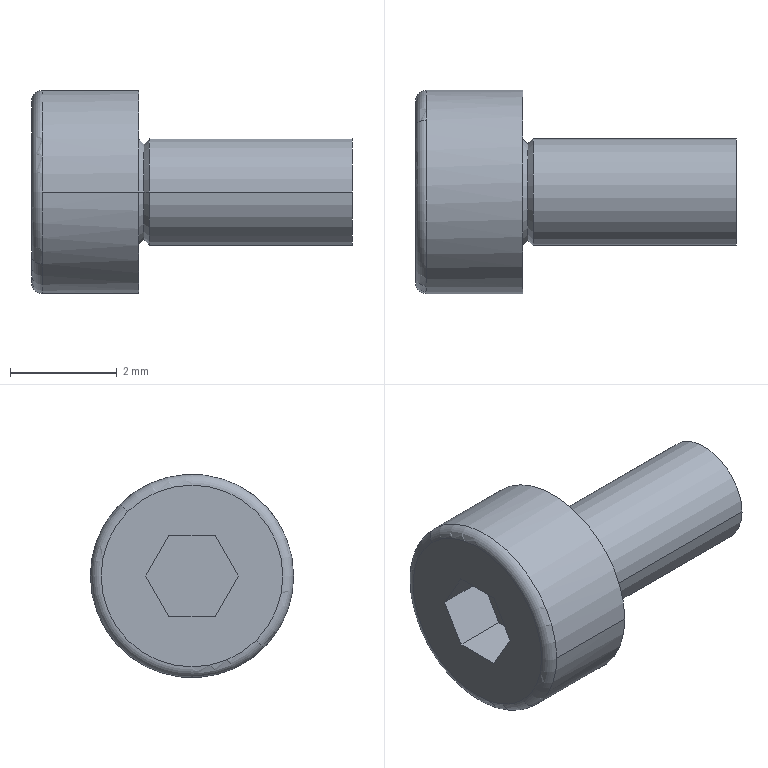Part | STEP file | ASND-0110-0211110210 | 1 solid | 20 faces | box 6 x 3.8 x 3.8 mm | volume 33.139 mm3 | plane 10 | cylinder 4 | cone 4 | torus 2 | commonest cylinder face diameters 2 x2 3.8 x2
STEP:
#1=CARTESIAN_POINT('',(0.,0.,0.));
#2=DIRECTION('',(0.,0.,1.));
#3=DIRECTION('',(1.,0.,0.));
#4=AXIS2_PLACEMENT_3D('',#1,#2,#3);
#5=CARTESIAN_POINT('',(-2.,-1.202,-1.202));
#6=VERTEX_POINT('',#5);
#7=CARTESIAN_POINT('',(-2.,1.202,1.202));
#8=VERTEX_POINT('',#7);
#9=CARTESIAN_POINT('',(-2.,0.,0.));
#10=DIRECTION('',(-1.,0.,0.));
#11=DIRECTION('',(0.,-1.,0.));
#12=AXIS2_PLACEMENT_3D('',#9,#10,#11);
#13=CIRCLE('',#12,1.7);
#14=CARTESIAN_POINT('',(-1.8,0.,0.));
#15=DIRECTION('',(1.,0.,0.));
#16=DIRECTION('',(0.,0.7071,0.7071));
#17=AXIS2_PLACEMENT_3D('',#14,#15,#16);
#18=TOROIDAL_SURFACE('',#17,1.7,0.2);
#19=CARTESIAN_POINT('',(8.639,4.712));
#20=DIRECTION('',(-1.,0.));
#21=VECTOR('',#20,1.);
#22=LINE('',#19,#21);
#23=(GEOMETRIC_REPRESENTATION_CONTEXT(2)PARAMETRIC_REPRESENTATION_CONTEXT()REPRESENTATION_CONTEXT('',''));
#24=DEFINITIONAL_REPRESENTATION('',(#22),#23);
#25=PCURVE('',#18,#24);
#26=CARTESIAN_POINT('',(-2.,0.,0.));
#27=DIRECTION('',(1.,0.,0.));
#28=DIRECTION('',(0.,0.7071,0.7071));
#29=AXIS2_PLACEMENT_3D('',#26,#27,#28);
#30=PLANE('',#29);
#31=CARTESIAN_POINT('',(-1.202,1.202));
#32=CARTESIAN_POINT('',(0.88,3.284));
#33=CARTESIAN_POINT('',(1.642,0.44));
#34=CARTESIAN_POINT('',(2.404,-2.404));
#35=CARTESIAN_POINT('',(-0.44,-1.642));
#36=CARTESIAN_POINT('',(-3.284,-0.88));
#37=CARTESIAN_POINT('',(-1.202,1.202));
#38=(BOUNDED_CURVE()B_SPLINE_CURVE(2,(#31,#32,#33,#34,#35,#36,#37),.UNSPECIFIED.,.T.,.F.)B_SPLINE_CURVE_WITH_KNOTS((1,2,2,2,2,1),(-2.094,0.,2.094,4.189,6.283,8.378),.UNSPECIFIED.)CURVE()GEOMETRIC_REPRESENTATION_ITEM()RATIONAL_B_SPLINE_CURVE((1.,0.5,1.,0.5,1.,0.5,1.))REPRESENTATION_ITEM(''));
#39=(GEOMETRIC_REPRESENTATION_CONTEXT(2)PARAMETRIC_REPRESENTATION_CONTEXT()REPRESENTATION_CONTEXT('',''));
#40=DEFINITIONAL_REPRESENTATION('',(#38),#39);
#41=PCURVE('',#30,#40);
#42=SURFACE_CURVE('',#13,(#25,#41),.PCURVE_S1.);
#43=EDGE_CURVE('',#6,#8,#42,.T.);
#44=ORIENTED_EDGE('',*,*,#43,.F.);
#45=CARTESIAN_POINT('',(-1.8,-1.344,-1.344));
#46=VERTEX_POINT('',#45);
#47=CARTESIAN_POINT('',(-1.8,-1.202,-1.202));
#48=DIRECTION('',(0.,-0.7071,0.7071));
#49=DIRECTION('',(0.,-0.7071,-0.7071));
#50=AXIS2_PLACEMENT_3D('',#47,#48,#49);
#51=CIRCLE('',#50,0.2);
#52=CARTESIAN_POINT('',(3.142,0.));
#53=DIRECTION('',(0.,1.));
#54=VECTOR('',#53,1.);
#55=LINE('',#52,#54);
#56=(GEOMETRIC_REPRESENTATION_CONTEXT(2)PARAMETRIC_REPRESENTATION_CONTEXT()REPRESENTATION_CONTEXT('',''));
#57=DEFINITIONAL_REPRESENTATION('',(#55),#56);
#58=PCURVE('',#18,#57);
#59=CARTESIAN_POINT('',(-1.8,0.,0.));
#60=DIRECTION('',(1.,0.,0.));
#61=DIRECTION('',(0.,0.7071,0.7071));
#62=AXIS2_PLACEMENT_3D('',#59,#60,#61);
#63=TOROIDAL_SURFACE('',#62,1.7,0.2);
#64=CARTESIAN_POINT('',(3.142,0.));
#65=DIRECTION('',(0.,1.));
#66=VECTOR('',#65,1.);
#67=LINE('',#64,#66);
#68=(GEOMETRIC_REPRESENTATION_CONTEXT(2)PARAMETRIC_REPRESENTATION_CONTEXT()REPRESENTATION_CONTEXT('',''));
#69=DEFINITIONAL_REPRESENTATION('',(#67),#68);
#70=PCURVE('',#63,#69);
#71=SURFACE_CURVE('',#51,(#58,#70),.PCURVE_S1.);
#72=EDGE_CURVE('',#6,#46,#71,.T.);
#73=ORIENTED_EDGE('',*,*,#72,.T.);
#74=CARTESIAN_POINT('',(-1.8,-1.9,0.));
#75=VERTEX_POINT('',#74);
#76=CARTESIAN_POINT('',(-1.8,0.,0.));
#77=DIRECTION('',(-1.,0.,0.));
#78=DIRECTION('',(0.,-1.,0.));
#79=AXIS2_PLACEMENT_3D('',#76,#77,#78);
#80=CIRCLE('',#79,1.9);
#81=CARTESIAN_POINT('',(8.639,6.283));
#82=DIRECTION('',(-1.,0.));
#83=VECTOR('',#82,1.);
#84=LINE('',#81,#83);
#85=(GEOMETRIC_REPRESENTATION_CONTEXT(2)PARAMETRIC_REPRESENTATION_CONTEXT()REPRESENTATION_CONTEXT('',''));
#86=DEFINITIONAL_REPRESENTATION('',(#84),#85);
#87=PCURVE('',#18,#86);
#88=CARTESIAN_POINT('',(-2.3,0.,0.));
#89=DIRECTION('',(1.,0.,0.));
#90=DIRECTION('',(0.,1.,0.));
#91=AXIS2_PLACEMENT_3D('',#88,#89,#90);
#92=CYLINDRICAL_SURFACE('',#91,1.9);
#93=CARTESIAN_POINT('',(9.425,0.5));
#94=DIRECTION('',(-1.,0.));
#95=VECTOR('',#94,1.);
#96=LINE('',#93,#95);
#97=(GEOMETRIC_REPRESENTATION_CONTEXT(2)PARAMETRIC_REPRESENTATION_CONTEXT()REPRESENTATION_CONTEXT('',''));
#98=DEFINITIONAL_REPRESENTATION('',(#96),#97);
#99=PCURVE('',#92,#98);
#100=SURFACE_CURVE('',#80,(#87,#99),.PCURVE_S1.);
#101=EDGE_CURVE('',#46,#75,#100,.T.);
#102=ORIENTED_EDGE('',*,*,#101,.T.);
#103=CARTESIAN_POINT('',(-1.8,1.344,1.344));
#104=VERTEX_POINT('',#103);
#105=CARTESIAN_POINT('',(-1.8,0.,0.));
#106=DIRECTION('',(-1.,0.,0.));
#107=DIRECTION('',(0.,-1.,0.));
#108=AXIS2_PLACEMENT_3D('',#105,#106,#107);
#109=CIRCLE('',#108,1.9);
#110=CARTESIAN_POINT('',(2.356,6.283));
#111=DIRECTION('',(-1.,0.));
#112=VECTOR('',#111,1.);
#113=LINE('',#110,#112);
#114=(GEOMETRIC_REPRESENTATION_CONTEXT(2)PARAMETRIC_REPRESENTATION_CONTEXT()REPRESENTATION_CONTEXT('',''));
#115=DEFINITIONAL_REPRESENTATION('',(#113),#114);
#116=PCURVE('',#18,#115);
#117=CARTESIAN_POINT('',(-2.3,0.,0.));
#118=DIRECTION('',(1.,0.,0.));
#119=DIRECTION('',(0.,1.,0.));
#120=AXIS2_PLACEMENT_3D('',#117,#118,#119);
#121=CYLINDRICAL_SURFACE('',#120,1.9);
#122=CARTESIAN_POINT('',(3.142,0.5));
#123=DIRECTION('',(-1.,0.));
#124=VECTOR('',#123,1.);
#125=LINE('',#122,#124);
#126=(GEOMETRIC_REPRESENTATION_CONTEXT(2)PARAMETRIC_REPRESENTATION_CONTEXT()REPRESENTATION_CONTEXT('',''));
#127=DEFINITIONAL_REPRESENTATION('',(#125),#126);
#128=PCURVE('',#121,#127);
#129=SURFACE_CURVE('',#109,(#116,#128),.PCURVE_S1.);
#130=EDGE_CURVE('',#75,#104,#129,.T.);
#131=ORIENTED_EDGE('',*,*,#130,.T.);
#132=CARTESIAN_POINT('',(-1.8,1.202,1.202));
#133=DIRECTION('',(0.,0.7071,-0.7071));
#134=DIRECTION('',(0.,0.7071,0.7071));
#135=AXIS2_PLACEMENT_3D('',#132,#133,#134);
#136=CIRCLE('',#135,0.2);
#137=CARTESIAN_POINT('',(0.,0.));
#138=DIRECTION('',(0.,1.));
#139=VECTOR('',#138,1.);
#140=LINE('',#137,#139);
#141=(GEOMETRIC_REPRESENTATION_CONTEXT(2)PARAMETRIC_REPRESENTATION_CONTEXT()REPRESENTATION_CONTEXT('',''));
#142=DEFINITIONAL_REPRESENTATION('',(#140),#141);
#143=PCURVE('',#18,#142);
#144=CARTESIAN_POINT('',(6.283,0.));
#145=DIRECTION('',(0.,1.));
#146=VECTOR('',#145,1.);
#147=LINE('',#144,#146);
#148=(GEOMETRIC_REPRESENTATION_CONTEXT(2)PARAMETRIC_REPRESENTATION_CONTEXT()REPRESENTATION_CONTEXT('',''));
#149=DEFINITIONAL_REPRESENTATION('',(#147),#148);
#150=PCURVE('',#63,#149);
#151=SURFACE_CURVE('',#136,(#143,#150),.PCURVE_S1.);
#152=EDGE_CURVE('',#8,#104,#151,.T.);
#153=ORIENTED_EDGE('',*,*,#152,.F.);
#154=EDGE_LOOP('',(#44,#73,#102,#131,#153));
#155=FACE_BOUND('',#154,.T.);
#156=ADVANCED_FACE('',(#155),#18,.T.);
#157=ORIENTED_EDGE('',*,*,#130,.F.);
#158=CARTESIAN_POINT('',(0.,-1.9,0.));
#159=VERTEX_POINT('',#158);
#160=CARTESIAN_POINT('',(-2.3,-1.9,0.));
#161=DIRECTION('',(1.,0.,0.));
#162=VECTOR('',#161,1.);
#163=LINE('',#160,#162);
#164=CARTESIAN_POINT('',(3.142,0.));
#165=DIRECTION('',(0.,1.));
#166=VECTOR('',#165,1.);
#167=LINE('',#164,#166);
#168=(GEOMETRIC_REPRESENTATION_CONTEXT(2)PARAMETRIC_REPRESENTATION_CONTEXT()REPRESENTATION_CONTEXT('',''));
#169=DEFINITIONAL_REPRESENTATION('',(#167),#168);
#170=PCURVE('',#121,#169);
#171=CARTESIAN_POINT('',(3.142,0.));
#172=DIRECTION('',(0.,1.));
#173=VECTOR('',#172,1.);
#174=LINE('',#171,#173);
#175=(GEOMETRIC_REPRESENTATION_CONTEXT(2)PARAMETRIC_REPRESENTATION_CONTEXT()REPRESENTATION_CONTEXT('',''));
#176=DEFINITIONAL_REPRESENTATION('',(#174),#175);
#177=PCURVE('',#92,#176);
#178=SURFACE_CURVE('',#163,(#170,#177),.PCURVE_S1.);
#179=EDGE_CURVE('',#75,#159,#178,.T.);
#180=ORIENTED_EDGE('',*,*,#179,.T.);
#181=CARTESIAN_POINT('',(0.,1.9,0.));
#182=VERTEX_POINT('',#181);
#183=CARTESIAN_POINT('',(0.,0.,0.));
#184=DIRECTION('',(-1.,0.,0.));
#185=DIRECTION('',(0.,-1.,0.));
#186=AXIS2_PLACEMENT_3D('',#183,#184,#185);
#187=CIRCLE('',#186,1.9);
#188=CARTESIAN_POINT('',(3.142,2.3));
#189=DIRECTION('',(-1.,0.));
#190=VECTOR('',#189,1.);
#191=LINE('',#188,#190);
#192=(GEOMETRIC_REPRESENTATION_CONTEXT(2)PARAMETRIC_REPRESENTATION_CONTEXT()REPRESENTATION_CONTEXT('',''));
#193=DEFINITIONAL_REPRESENTATION('',(#191),#192);
#194=PCURVE('',#121,#193);
#195=CARTESIAN_POINT('',(0.,0.,0.));
#196=DIRECTION('',(1.,0.,0.));
#197=DIRECTION('',(0.,0.7071,0.7071));
#198=AXIS2_PLACEMENT_3D('',#195,#196,#197);
#199=PLANE('',#198);
#200=CARTESIAN_POINT('',(-1.344,1.344));
#201=CARTESIAN_POINT('',(0.9835,3.671));
#202=CARTESIAN_POINT('',(1.835,0.4918));
#203=CARTESIAN_POINT('',(2.687,-2.687));
#204=CARTESIAN_POINT('',(-0.4918,-1.835));
#205=CARTESIAN_POINT('',(-3.671,-0.9835));
#206=CARTESIAN_POINT('',(-1.344,1.344));
#207=(BOUNDED_CURVE()B_SPLINE_CURVE(2,(#200,#201,#202,#203,#204,#205,#206),.UNSPECIFIED.,.T.,.F.)B_SPLINE_CURVE_WITH_KNOTS((1,2,2,2,2,1),(-2.094,0.,2.094,4.189,6.283,8.378),.UNSPECIFIED.)CURVE()GEOMETRIC_REPRESENTATION_ITEM()RATIONAL_B_SPLINE_CURVE((1.,0.5,1.,0.5,1.,0.5,1.))REPRESENTATION_ITEM(''));
#208=(GEOMETRIC_REPRESENTATION_CONTEXT(2)PARAMETRIC_REPRESENTATION_CONTEXT()REPRESENTATION_CONTEXT('',''));
#209=DEFINITIONAL_REPRESENTATION('',(#207),#208);
#210=PCURVE('',#199,#209);
#211=SURFACE_CURVE('',#187,(#194,#210),.PCURVE_S1.);
#212=EDGE_CURVE('',#159,#182,#211,.T.);
#213=ORIENTED_EDGE('',*,*,#212,.T.);
#214=CARTESIAN_POINT('',(-1.8,1.9,0.));
#215=VERTEX_POINT('',#214);
#216=CARTESIAN_POINT('',(-2.3,1.9,0.));
#217=DIRECTION('',(1.,0.,0.));
#218=VECTOR('',#217,1.);
#219=LINE('',#216,#218);
#220=CARTESIAN_POINT('',(0.,0.));
#221=DIRECTION('',(0.,1.));
#222=VECTOR('',#221,1.);
#223=LINE('',#220,#222);
#224=(GEOMETRIC_REPRESENTATION_CONTEXT(2)PARAMETRIC_REPRESENTATION_CONTEXT()REPRESENTATION_CONTEXT('',''));
#225=DEFINITIONAL_REPRESENTATION('',(#223),#224);
#226=PCURVE('',#121,#225);
#227=CARTESIAN_POINT('',(6.283,0.));
#228=DIRECTION('',(0.,1.));
#229=VECTOR('',#228,1.);
#230=LINE('',#227,#229);
#231=(GEOMETRIC_REPRESENTATION_CONTEXT(2)PARAMETRIC_REPRESENTATION_CONTEXT()REPRESENTATION_CONTEXT('',''));
#232=DEFINITIONAL_REPRESENTATION('',(#230),#231);
#233=PCURVE('',#92,#232);
#234=SURFACE_CURVE('',#219,(#226,#233),.PCURVE_S1.);
#235=EDGE_CURVE('',#215,#182,#234,.T.);
#236=ORIENTED_EDGE('',*,*,#235,.F.);
#237=CARTESIAN_POINT('',(-1.8,0.,0.));
#238=DIRECTION('',(-1.,0.,0.));
#239=DIRECTION('',(0.,-1.,0.));
#240=AXIS2_PLACEMENT_3D('',#237,#238,#239);
#241=CIRCLE('',#240,1.9);
#242=CARTESIAN_POINT('',(3.142,0.5));
#243=DIRECTION('',(-1.,0.));
#244=VECTOR('',#243,1.);
#245=LINE('',#242,#244);
#246=(GEOMETRIC_REPRESENTATION_CONTEXT(2)PARAMETRIC_REPRESENTATION_CONTEXT()REPRESENTATION_CONTEXT('',''));
#247=DEFINITIONAL_REPRESENTATION('',(#245),#246);
#248=PCURVE('',#121,#247);
#249=CARTESIAN_POINT('',(8.639,6.283));
#250=DIRECTION('',(-1.,0.));
#251=VECTOR('',#250,1.);
#252=LINE('',#249,#251);
#253=(GEOMETRIC_REPRESENTATION_CONTEXT(2)PARAMETRIC_REPRESENTATION_CONTEXT()REPRESENTATION_CONTEXT('',''));
#254=DEFINITIONAL_REPRESENTATION('',(#252),#253);
#255=PCURVE('',#63,#254);
#256=SURFACE_CURVE('',#241,(#248,#255),.PCURVE_S1.);
#257=EDGE_CURVE('',#104,#215,#256,.T.);
#258=ORIENTED_EDGE('',*,*,#257,.F.);
#259=EDGE_LOOP('',(#157,#180,#213,#236,#258));
#260=FACE_BOUND('',#259,.T.);
#261=ADVANCED_FACE('',(#260),#121,.T.);
#262=CARTESIAN_POINT('',(0.1,-0.9,0.));
#263=VERTEX_POINT('',#262);
#264=CARTESIAN_POINT('',(0.1,0.9,0.));
#265=VERTEX_POINT('',#264);
#266=CARTESIAN_POINT('',(0.1,0.,0.));
#267=DIRECTION('',(1.,0.,0.));
#268=DIRECTION('',(0.,1.,0.));
#269=AXIS2_PLACEMENT_3D('',#266,#267,#268);
#270=CIRCLE('',#269,0.9);
#271=CARTESIAN_POINT('',(0.,0.,0.));
#272=DIRECTION('',(-1.,0.,0.));
#273=DIRECTION('',(0.,1.,0.));
#274=AXIS2_PLACEMENT_3D('',#271,#272,#273);
#275=CONICAL_SURFACE('',#274,1.,0.7854);
#276=CARTESIAN_POINT('',(6.283,-0.1));
#277=DIRECTION('',(-1.,0.));
#278=VECTOR('',#277,1.);
#279=LINE('',#276,#278);
#280=(GEOMETRIC_REPRESENTATION_CONTEXT(2)PARAMETRIC_REPRESENTATION_CONTEXT()REPRESENTATION_CONTEXT('',''));
#281=DEFINITIONAL_REPRESENTATION('',(#279),#280);
#282=PCURVE('',#275,#281);
#283=CARTESIAN_POINT('',(0.2,0.,0.));
#284=DIRECTION('',(1.,0.,0.));
#285=DIRECTION('',(0.,-1.,0.));
#286=AXIS2_PLACEMENT_3D('',#283,#284,#285);
#287=CONICAL_SURFACE('',#286,1.,0.7854);
#288=CARTESIAN_POINT('',(-3.142,-0.1));
#289=DIRECTION('',(1.,0.));
#290=VECTOR('',#289,1.);
#291=LINE('',#288,#290);
#292=(GEOMETRIC_REPRESENTATION_CONTEXT(2)PARAMETRIC_REPRESENTATION_CONTEXT()REPRESENTATION_CONTEXT('',''));
#293=DEFINITIONAL_REPRESENTATION('',(#291),#292);
#294=PCURVE('',#287,#293);
#295=SURFACE_CURVE('',#270,(#282,#294),.PCURVE_S1.);
#296=EDGE_CURVE('',#263,#265,#295,.T.);
#297=ORIENTED_EDGE('',*,*,#296,.F.);
#298=CARTESIAN_POINT('',(0.,-1.,0.));
#299=VERTEX_POINT('',#298);
#300=CARTESIAN_POINT('',(0.,-1.,0.));
#301=DIRECTION('',(-0.7071,-0.7071,0.));
#302=VECTOR('',#301,1.);
#303=LINE('',#300,#302);
#304=CARTESIAN_POINT('',(3.142,0.));
#305=DIRECTION('',(0.,1.));
#306=VECTOR('',#305,1.);
#307=LINE('',#304,#306);
#308=(GEOMETRIC_REPRESENTATION_CONTEXT(2)PARAMETRIC_REPRESENTATION_CONTEXT()REPRESENTATION_CONTEXT('',''));
#309=DEFINITIONAL_REPRESENTATION('',(#307),#308);
#310=PCURVE('',#275,#309);
#311=CARTESIAN_POINT('',(0.,0.,0.));
#312=DIRECTION('',(-1.,0.,0.));
#313=DIRECTION('',(0.,1.,0.));
#314=AXIS2_PLACEMENT_3D('',#311,#312,#313);
#315=CONICAL_SURFACE('',#314,1.,0.7854);
#316=CARTESIAN_POINT('',(3.142,0.));
#317=DIRECTION('',(0.,1.));
#318=VECTOR('',#317,1.);
#319=LINE('',#316,#318);
#320=(GEOMETRIC_REPRESENTATION_CONTEXT(2)PARAMETRIC_REPRESENTATION_CONTEXT()REPRESENTATION_CONTEXT('',''));
#321=DEFINITIONAL_REPRESENTATION('',(#319),#320);
#322=PCURVE('',#315,#321);
#323=SURFACE_CURVE('',#303,(#310,#322),.PCURVE_S1.);
#324=EDGE_CURVE('',#263,#299,#323,.T.);
#325=ORIENTED_EDGE('',*,*,#324,.T.);
#326=CARTESIAN_POINT('',(0.,1.,0.));
#327=VERTEX_POINT('',#326);
#328=CARTESIAN_POINT('',(0.,0.,0.));
#329=DIRECTION('',(1.,0.,0.));
#330=DIRECTION('',(0.,-1.,0.));
#331=AXIS2_PLACEMENT_3D('',#328,#329,#330);
#332=CIRCLE('',#331,1.);
#333=CARTESIAN_POINT('',(3.142,0.));
#334=DIRECTION('',(-1.,0.));
#335=VECTOR('',#334,1.);
#336=LINE('',#333,#335);
#337=(GEOMETRIC_REPRESENTATION_CONTEXT(2)PARAMETRIC_REPRESENTATION_CONTEXT()REPRESENTATION_CONTEXT('',''));
#338=DEFINITIONAL_REPRESENTATION('',(#336),#337);
#339=PCURVE('',#275,#338);
#340=CARTESIAN_POINT('',(0.,0.));
#341=DIRECTION('',(-0.7071,0.7071));
#342=AXIS2_PLACEMENT_2D('',#340,#341);
#343=CIRCLE('',#342,1.);
#344=(GEOMETRIC_REPRESENTATION_CONTEXT(2)PARAMETRIC_REPRESENTATION_CONTEXT()REPRESENTATION_CONTEXT('',''));
#345=DEFINITIONAL_REPRESENTATION('',(#343),#344);
#346=PCURVE('',#199,#345);
#347=SURFACE_CURVE('',#332,(#339,#346),.PCURVE_S1.);
#348=EDGE_CURVE('',#299,#327,#347,.T.);
#349=ORIENTED_EDGE('',*,*,#348,.T.);
#350=CARTESIAN_POINT('',(0.,1.,0.));
#351=DIRECTION('',(-0.7071,0.7071,0.));
#352=VECTOR('',#351,1.);
#353=LINE('',#350,#352);
#354=CARTESIAN_POINT('',(0.,0.));
#355=DIRECTION('',(0.,1.));
#356=VECTOR('',#355,1.);
#357=LINE('',#354,#356);
#358=(GEOMETRIC_REPRESENTATION_CONTEXT(2)PARAMETRIC_REPRESENTATION_CONTEXT()REPRESENTATION_CONTEXT('',''));
#359=DEFINITIONAL_REPRESENTATION('',(#357),#358);
#360=PCURVE('',#275,#359);
#361=CARTESIAN_POINT('',(6.283,0.));
#362=DIRECTION('',(0.,1.));
#363=VECTOR('',#362,1.);
#364=LINE('',#361,#363);
#365=(GEOMETRIC_REPRESENTATION_CONTEXT(2)PARAMETRIC_REPRESENTATION_CONTEXT()REPRESENTATION_CONTEXT('',''));
#366=DEFINITIONAL_REPRESENTATION('',(#364),#365);
#367=PCURVE('',#315,#366);
#368=SURFACE_CURVE('',#353,(#360,#367),.PCURVE_S1.);
#369=EDGE_CURVE('',#265,#327,#368,.T.);
#370=ORIENTED_EDGE('',*,*,#369,.F.);
#371=EDGE_LOOP('',(#297,#325,#349,#370));
#372=FACE_BOUND('',#371,.T.);
#373=ADVANCED_FACE('',(#372),#275,.T.);
#374=ORIENTED_EDGE('',*,*,#296,.T.);
#375=CARTESIAN_POINT('',(0.2,1.,0.));
#376=VERTEX_POINT('',#375);
#377=CARTESIAN_POINT('',(0.2,1.,0.));
#378=DIRECTION('',(0.7071,0.7071,0.));
#379=VECTOR('',#378,1.);
#380=LINE('',#377,#379);
#381=CARTESIAN_POINT('',(3.142,0.));
#382=DIRECTION('',(0.,1.));
#383=VECTOR('',#382,1.);
#384=LINE('',#381,#383);
#385=(GEOMETRIC_REPRESENTATION_CONTEXT(2)PARAMETRIC_REPRESENTATION_CONTEXT()REPRESENTATION_CONTEXT('',''));
#386=DEFINITIONAL_REPRESENTATION('',(#384),#385);
#387=PCURVE('',#287,#386);
#388=CARTESIAN_POINT('',(0.2,0.,0.));
#389=DIRECTION('',(1.,0.,0.));
#390=DIRECTION('',(0.,-1.,0.));
#391=AXIS2_PLACEMENT_3D('',#388,#389,#390);
#392=CONICAL_SURFACE('',#391,1.,0.7854);
#393=CARTESIAN_POINT('',(3.142,0.));
#394=DIRECTION('',(0.,1.));
#395=VECTOR('',#394,1.);
#396=LINE('',#393,#395);
#397=(GEOMETRIC_REPRESENTATION_CONTEXT(2)PARAMETRIC_REPRESENTATION_CONTEXT()REPRESENTATION_CONTEXT('',''));
#398=DEFINITIONAL_REPRESENTATION('',(#396),#397);
#399=PCURVE('',#392,#398);
#400=SURFACE_CURVE('',#380,(#387,#399),.PCURVE_S1.);
#401=EDGE_CURVE('',#265,#376,#400,.T.);
#402=ORIENTED_EDGE('',*,*,#401,.T.);
#403=CARTESIAN_POINT('',(0.2,-1.,0.));
#404=VERTEX_POINT('',#403);
#405=CARTESIAN_POINT('',(0.2,0.,0.));
#406=DIRECTION('',(1.,0.,0.));
#407=DIRECTION('',(0.,1.,0.));
#408=AXIS2_PLACEMENT_3D('',#405,#406,#407);
#409=CIRCLE('',#408,1.);
#410=CARTESIAN_POINT('',(-3.142,0.));
#411=DIRECTION('',(1.,0.));
#412=VECTOR('',#411,1.);
#413=LINE('',#410,#412);
#414=(GEOMETRIC_REPRESENTATION_CONTEXT(2)PARAMETRIC_REPRESENTATION_CONTEXT()REPRESENTATION_CONTEXT('',''));
#415=DEFINITIONAL_REPRESENTATION('',(#413),#414);
#416=PCURVE('',#287,#415);
#417=CARTESIAN_POINT('',(-2.3,0.,0.));
#418=DIRECTION('',(1.,0.,0.));
#419=DIRECTION('',(0.,1.,0.));
#420=AXIS2_PLACEMENT_3D('',#417,#418,#419);
#421=CYLINDRICAL_SURFACE('',#420,1.);
#422=CARTESIAN_POINT('',(0.,2.5));
#423=DIRECTION('',(1.,0.));
#424=VECTOR('',#423,1.);
#425=LINE('',#422,#424);
#426=(GEOMETRIC_REPRESENTATION_CONTEXT(2)PARAMETRIC_REPRESENTATION_CONTEXT()REPRESENTATION_CONTEXT('',''));
#427=DEFINITIONAL_REPRESENTATION('',(#425),#426);
#428=PCURVE('',#421,#427);
#429=SURFACE_CURVE('',#409,(#416,#428),.PCURVE_S1.);
#430=EDGE_CURVE('',#404,#376,#429,.T.);
#431=ORIENTED_EDGE('',*,*,#430,.F.);
#432=CARTESIAN_POINT('',(0.2,-1.,0.));
#433=DIRECTION('',(0.7071,-0.7071,0.));
#434=VECTOR('',#433,1.);
#435=LINE('',#432,#434);
#436=CARTESIAN_POINT('',(0.,0.));
#437=DIRECTION('',(0.,1.));
#438=VECTOR('',#437,1.);
#439=LINE('',#436,#438);
#440=(GEOMETRIC_REPRESENTATION_CONTEXT(2)PARAMETRIC_REPRESENTATION_CONTEXT()REPRESENTATION_CONTEXT('',''));
#441=DEFINITIONAL_REPRESENTATION('',(#439),#440);
#442=PCURVE('',#287,#441);
#443=CARTESIAN_POINT('',(6.283,0.));
#444=DIRECTION('',(0.,1.));
#445=VECTOR('',#444,1.);
#446=LINE('',#443,#445);
#447=(GEOMETRIC_REPRESENTATION_CONTEXT(2)PARAMETRIC_REPRESENTATION_CONTEXT()REPRESENTATION_CONTEXT('',''));
#448=DEFINITIONAL_REPRESENTATION('',(#446),#447);
#449=PCURVE('',#392,#448);
#450=SURFACE_CURVE('',#435,(#442,#449),.PCURVE_S1.);
#451=EDGE_CURVE('',#263,#404,#450,.T.);
#452=ORIENTED_EDGE('',*,*,#451,.F.);
#453=EDGE_LOOP('',(#374,#402,#431,#452));
#454=FACE_BOUND('',#453,.T.);
#455=ADVANCED_FACE('',(#454),#287,.T.);
#456=CARTESIAN_POINT('',(0.2,0.,0.));
#457=DIRECTION('',(1.,0.,0.));
#458=DIRECTION('',(0.,1.,0.));
#459=AXIS2_PLACEMENT_3D('',#456,#457,#458);
#460=CIRCLE('',#459,1.);
#461=CARTESIAN_POINT('',(-2.3,0.,0.));
#462=DIRECTION('',(1.,0.,0.));
#463=DIRECTION('',(0.,1.,0.));
#464=AXIS2_PLACEMENT_3D('',#461,#462,#463);
#465=CYLINDRICAL_SURFACE('',#464,1.);
#466=CARTESIAN_POINT('',(0.,2.5));
#467=DIRECTION('',(1.,0.));
#468=VECTOR('',#467,1.);
#469=LINE('',#466,#468);
#470=(GEOMETRIC_REPRESENTATION_CONTEXT(2)PARAMETRIC_REPRESENTATION_CONTEXT()REPRESENTATION_CONTEXT('',''));
#471=DEFINITIONAL_REPRESENTATION('',(#469),#470);
#472=PCURVE('',#465,#471);
#473=CARTESIAN_POINT('',(3.142,0.));
#474=DIRECTION('',(1.,0.));
#475=VECTOR('',#474,1.);
#476=LINE('',#473,#475);
#477=(GEOMETRIC_REPRESENTATION_CONTEXT(2)PARAMETRIC_REPRESENTATION_CONTEXT()REPRESENTATION_CONTEXT('',''));
#478=DEFINITIONAL_REPRESENTATION('',(#476),#477);
#479=PCURVE('',#392,#478);
#480=SURFACE_CURVE('',#460,(#472,#479),.PCURVE_S1.);
#481=EDGE_CURVE('',#376,#404,#480,.T.);
#482=ORIENTED_EDGE('',*,*,#481,.T.);
#483=CARTESIAN_POINT('',(4.,-1.,0.));
#484=VERTEX_POINT('',#483);
#485=CARTESIAN_POINT('',(-2.3,-1.,0.));
#486=DIRECTION('',(1.,0.,0.));
#487=VECTOR('',#486,1.);
#488=LINE('',#485,#487);
#489=CARTESIAN_POINT('',(3.142,0.));
#490=DIRECTION('',(0.,1.));
#491=VECTOR('',#490,1.);
#492=LINE('',#489,#491);
#493=(GEOMETRIC_REPRESENTATION_CONTEXT(2)PARAMETRIC_REPRESENTATION_CONTEXT()REPRESENTATION_CONTEXT('',''));
#494=DEFINITIONAL_REPRESENTATION('',(#492),#493);
#495=PCURVE('',#465,#494);
#496=CARTESIAN_POINT('',(3.142,0.));
#497=DIRECTION('',(0.,1.));
#498=VECTOR('',#497,1.);
#499=LINE('',#496,#498);
#500=(GEOMETRIC_REPRESENTATION_CONTEXT(2)PARAMETRIC_REPRESENTATION_CONTEXT()REPRESENTATION_CONTEXT('',''));
#501=DEFINITIONAL_REPRESENTATION('',(#499),#500);
#502=PCURVE('',#421,#501);
#503=SURFACE_CURVE('',#488,(#495,#502),.PCURVE_S1.);
#504=EDGE_CURVE('',#404,#484,#503,.T.);
#505=ORIENTED_EDGE('',*,*,#504,.T.);
#506=CARTESIAN_POINT('',(4.,1.,0.));
#507=VERTEX_POINT('',#506);
#508=CARTESIAN_POINT('',(4.,0.,0.));
#509=DIRECTION('',(-1.,0.,0.));
#510=DIRECTION('',(0.,-1.,0.));
#511=AXIS2_PLACEMENT_3D('',#508,#509,#510);
#512=CIRCLE('',#511,1.);
#513=CARTESIAN_POINT('',(3.142,6.3));
#514=DIRECTION('',(-1.,0.));
#515=VECTOR('',#514,1.);
#516=LINE('',#513,#515);
#517=(GEOMETRIC_REPRESENTATION_CONTEXT(2)PARAMETRIC_REPRESENTATION_CONTEXT()REPRESENTATION_CONTEXT('',''));
#518=DEFINITIONAL_REPRESENTATION('',(#516),#517);
#519=PCURVE('',#465,#518);
#520=CARTESIAN_POINT('',(4.,0.,0.));
#521=DIRECTION('',(1.,0.,0.));
#522=DIRECTION('',(0.,0.7071,0.7071));
#523=AXIS2_PLACEMENT_3D('',#520,#521,#522);
#524=PLANE('',#523);
#525=CARTESIAN_POINT('',(-0.7071,0.7071));
#526=CARTESIAN_POINT('',(0.5176,1.932));
#527=CARTESIAN_POINT('',(0.9659,0.2588));
#528=CARTESIAN_POINT('',(1.414,-1.414));
#529=CARTESIAN_POINT('',(-0.2588,-0.9659));
#530=CARTESIAN_POINT('',(-1.932,-0.5176));
#531=CARTESIAN_POINT('',(-0.7071,0.7071));
#532=(BOUNDED_CURVE()B_SPLINE_CURVE(2,(#525,#526,#527,#528,#529,#530,#531),.UNSPECIFIED.,.T.,.F.)B_SPLINE_CURVE_WITH_KNOTS((1,2,2,2,2,1),(-2.094,0.,2.094,4.189,6.283,8.378),.UNSPECIFIED.)CURVE()GEOMETRIC_REPRESENTATION_ITEM()RATIONAL_B_SPLINE_CURVE((1.,0.5,1.,0.5,1.,0.5,1.))REPRESENTATION_ITEM(''));
#533=(GEOMETRIC_REPRESENTATION_CONTEXT(2)PARAMETRIC_REPRESENTATION_CONTEXT()REPRESENTATION_CONTEXT('',''));
#534=DEFINITIONAL_REPRESENTATION('',(#532),#533);
#535=PCURVE('',#524,#534);
#536=SURFACE_CURVE('',#512,(#519,#535),.PCURVE_S1.);
#537=EDGE_CURVE('',#484,#507,#536,.T.);
#538=ORIENTED_EDGE('',*,*,#537,.T.);
#539=CARTESIAN_POINT('',(-2.3,1.,0.));
#540=DIRECTION('',(1.,0.,0.));
#541=VECTOR('',#540,1.);
#542=LINE('',#539,#541);
#543=CARTESIAN_POINT('',(0.,0.));
#544=DIRECTION('',(0.,1.));
#545=VECTOR('',#544,1.);
#546=LINE('',#543,#545);
#547=(GEOMETRIC_REPRESENTATION_CONTEXT(2)PARAMETRIC_REPRESENTATION_CONTEXT()REPRESENTATION_CONTEXT('',''));
#548=DEFINITIONAL_REPRESENTATION('',(#546),#547);
#549=PCURVE('',#465,#548);
#550=CARTESIAN_POINT('',(6.283,0.));
#551=DIRECTION('',(0.,1.));
#552=VECTOR('',#551,1.);
#553=LINE('',#550,#552);
#554=(GEOMETRIC_REPRESENTATION_CONTEXT(2)PARAMETRIC_REPRESENTATION_CONTEXT()REPRESENTATION_CONTEXT('',''));
#555=DEFINITIONAL_REPRESENTATION('',(#553),#554);
#556=PCURVE('',#421,#555);
#557=SURFACE_CURVE('',#542,(#549,#556),.PCURVE_S1.);
#558=EDGE_CURVE('',#376,#507,#557,.T.);
#559=ORIENTED_EDGE('',*,*,#558,.F.);
#560=EDGE_LOOP('',(#482,#505,#538,#559));
#561=FACE_BOUND('',#560,.T.);
#562=ADVANCED_FACE('',(#561),#465,.T.);
#563=CARTESIAN_POINT('',(4.,0.,0.));
#564=DIRECTION('',(-1.,0.,0.));
#565=DIRECTION('',(0.,-1.,0.));
#566=AXIS2_PLACEMENT_3D('',#563,#564,#565);
#567=CIRCLE('',#566,1.);
#568=CARTESIAN_POINT('',(-0.7071,0.7071));
#569=CARTESIAN_POINT('',(0.5176,1.932));
#570=CARTESIAN_POINT('',(0.9659,0.2588));
#571=CARTESIAN_POINT('',(1.414,-1.414));
#572=CARTESIAN_POINT('',(-0.2588,-0.9659));
#573=CARTESIAN_POINT('',(-1.932,-0.5176));
#574=CARTESIAN_POINT('',(-0.7071,0.7071));
#575=(BOUNDED_CURVE()B_SPLINE_CURVE(2,(#568,#569,#570,#571,#572,#573,#574),.UNSPECIFIED.,.T.,.F.)B_SPLINE_CURVE_WITH_KNOTS((1,2,2,2,2,1),(-2.094,0.,2.094,4.189,6.283,8.378),.UNSPECIFIED.)CURVE()GEOMETRIC_REPRESENTATION_ITEM()RATIONAL_B_SPLINE_CURVE((1.,0.5,1.,0.5,1.,0.5,1.))REPRESENTATION_ITEM(''));
#576=(GEOMETRIC_REPRESENTATION_CONTEXT(2)PARAMETRIC_REPRESENTATION_CONTEXT()REPRESENTATION_CONTEXT('',''));
#577=DEFINITIONAL_REPRESENTATION('',(#575),#576);
#578=PCURVE('',#524,#577);
#579=CARTESIAN_POINT('',(9.425,6.3));
#580=DIRECTION('',(-1.,0.));
#581=VECTOR('',#580,1.);
#582=LINE('',#579,#581);
#583=(GEOMETRIC_REPRESENTATION_CONTEXT(2)PARAMETRIC_REPRESENTATION_CONTEXT()REPRESENTATION_CONTEXT('',''));
#584=DEFINITIONAL_REPRESENTATION('',(#582),#583);
#585=PCURVE('',#421,#584);
#586=SURFACE_CURVE('',#567,(#578,#585),.PCURVE_S1.);
#587=EDGE_CURVE('',#507,#484,#586,.T.);
#588=ORIENTED_EDGE('',*,*,#587,.F.);
#589=ORIENTED_EDGE('',*,*,#537,.F.);
#590=EDGE_LOOP('',(#588,#589));
#591=FACE_BOUND('',#590,.T.);
#592=ADVANCED_FACE('',(#591),#524,.T.);
#593=ORIENTED_EDGE('',*,*,#504,.F.);
#594=ORIENTED_EDGE('',*,*,#430,.T.);
#595=ORIENTED_EDGE('',*,*,#558,.T.);
#596=ORIENTED_EDGE('',*,*,#587,.T.);
#597=EDGE_LOOP('',(#593,#594,#595,#596));
#598=FACE_BOUND('',#597,.T.);
#599=ADVANCED_FACE('',(#598),#421,.T.);
#600=ORIENTED_EDGE('',*,*,#401,.F.);
#601=CARTESIAN_POINT('',(0.1,0.,0.));
#602=DIRECTION('',(1.,0.,0.));
#603=DIRECTION('',(0.,1.,0.));
#604=AXIS2_PLACEMENT_3D('',#601,#602,#603);
#605=CIRCLE('',#604,0.9);
#606=CARTESIAN_POINT('',(3.142,-0.1));
#607=DIRECTION('',(1.,0.));
#608=VECTOR('',#607,1.);
#609=LINE('',#606,#608);
#610=(GEOMETRIC_REPRESENTATION_CONTEXT(2)PARAMETRIC_REPRESENTATION_CONTEXT()REPRESENTATION_CONTEXT('',''));
#611=DEFINITIONAL_REPRESENTATION('',(#609),#610);
#612=PCURVE('',#392,#611);
#613=CARTESIAN_POINT('',(6.283,-0.1));
#614=DIRECTION('',(-1.,0.));
#615=VECTOR('',#614,1.);
#616=LINE('',#613,#615);
#617=(GEOMETRIC_REPRESENTATION_CONTEXT(2)PARAMETRIC_REPRESENTATION_CONTEXT()REPRESENTATION_CONTEXT('',''));
#618=DEFINITIONAL_REPRESENTATION('',(#616),#617);
#619=PCURVE('',#315,#618);
#620=SURFACE_CURVE('',#605,(#612,#619),.PCURVE_S1.);
#621=EDGE_CURVE('',#265,#263,#620,.T.);
#622=ORIENTED_EDGE('',*,*,#621,.T.);
#623=ORIENTED_EDGE('',*,*,#451,.T.);
#624=ORIENTED_EDGE('',*,*,#481,.F.);
#625=EDGE_LOOP('',(#600,#622,#623,#624));
#626=FACE_BOUND('',#625,.T.);
#627=ADVANCED_FACE('',(#626),#392,.T.);
#628=ORIENTED_EDGE('',*,*,#324,.F.);
#629=ORIENTED_EDGE('',*,*,#621,.F.);
#630=ORIENTED_EDGE('',*,*,#369,.T.);
#631=CARTESIAN_POINT('',(0.,0.,0.));
#632=DIRECTION('',(1.,0.,0.));
#633=DIRECTION('',(0.,-1.,0.));
#634=AXIS2_PLACEMENT_3D('',#631,#632,#633);
#635=CIRCLE('',#634,1.);
#636=CARTESIAN_POINT('',(9.425,0.));
#637=DIRECTION('',(-1.,0.));
#638=VECTOR('',#637,1.);
#639=LINE('',#636,#638);
#640=(GEOMETRIC_REPRESENTATION_CONTEXT(2)PARAMETRIC_REPRESENTATION_CONTEXT()REPRESENTATION_CONTEXT('',''));
#641=DEFINITIONAL_REPRESENTATION('',(#639),#640);
#642=PCURVE('',#315,#641);
#643=CARTESIAN_POINT('',(0.,0.));
#644=DIRECTION('',(-0.7071,0.7071));
#645=AXIS2_PLACEMENT_2D('',#643,#644);
#646=CIRCLE('',#645,1.);
#647=(GEOMETRIC_REPRESENTATION_CONTEXT(2)PARAMETRIC_REPRESENTATION_CONTEXT()REPRESENTATION_CONTEXT('',''));
#648=DEFINITIONAL_REPRESENTATION('',(#646),#647);
#649=PCURVE('',#199,#648);
#650=SURFACE_CURVE('',#635,(#642,#649),.PCURVE_S1.);
#651=EDGE_CURVE('',#327,#299,#650,.T.);
#652=ORIENTED_EDGE('',*,*,#651,.T.);
#653=EDGE_LOOP('',(#628,#629,#630,#652));
#654=FACE_BOUND('',#653,.T.);
#655=ADVANCED_FACE('',(#654),#315,.T.);
#656=CARTESIAN_POINT('',(0.,0.,0.));
#657=DIRECTION('',(-1.,0.,0.));
#658=DIRECTION('',(0.,-1.,0.));
#659=AXIS2_PLACEMENT_3D('',#656,#657,#658);
#660=CIRCLE('',#659,1.9);
#661=CARTESIAN_POINT('',(-1.344,1.344));
#662=CARTESIAN_POINT('',(0.9835,3.671));
#663=CARTESIAN_POINT('',(1.835,0.4918));
#664=CARTESIAN_POINT('',(2.687,-2.687));
#665=CARTESIAN_POINT('',(-0.4918,-1.835));
#666=CARTESIAN_POINT('',(-3.671,-0.9835));
#667=CARTESIAN_POINT('',(-1.344,1.344));
#668=(BOUNDED_CURVE()B_SPLINE_CURVE(2,(#661,#662,#663,#664,#665,#666,#667),.UNSPECIFIED.,.T.,.F.)B_SPLINE_CURVE_WITH_KNOTS((1,2,2,2,2,1),(-2.094,0.,2.094,4.189,6.283,8.378),.UNSPECIFIED.)CURVE()GEOMETRIC_REPRESENTATION_ITEM()RATIONAL_B_SPLINE_CURVE((1.,0.5,1.,0.5,1.,0.5,1.))REPRESENTATION_ITEM(''));
#669=(GEOMETRIC_REPRESENTATION_CONTEXT(2)PARAMETRIC_REPRESENTATION_CONTEXT()REPRESENTATION_CONTEXT('',''));
#670=DEFINITIONAL_REPRESENTATION('',(#668),#669);
#671=PCURVE('',#199,#670);
#672=CARTESIAN_POINT('',(9.425,2.3));
#673=DIRECTION('',(-1.,0.));
#674=VECTOR('',#673,1.);
#675=LINE('',#672,#674);
#676=(GEOMETRIC_REPRESENTATION_CONTEXT(2)PARAMETRIC_REPRESENTATION_CONTEXT()REPRESENTATION_CONTEXT('',''));
#677=DEFINITIONAL_REPRESENTATION('',(#675),#676);
#678=PCURVE('',#92,#677);
#679=SURFACE_CURVE('',#660,(#671,#678),.PCURVE_S1.);
#680=EDGE_CURVE('',#182,#159,#679,.T.);
#681=ORIENTED_EDGE('',*,*,#680,.F.);
#682=ORIENTED_EDGE('',*,*,#212,.F.);
#683=EDGE_LOOP('',(#681,#682));
#684=FACE_BOUND('',#683,.T.);
#685=ORIENTED_EDGE('',*,*,#651,.F.);
#686=ORIENTED_EDGE('',*,*,#348,.F.);
#687=EDGE_LOOP('',(#685,#686));
#688=FACE_BOUND('',#687,.T.);
#689=ADVANCED_FACE('',(#684,#688),#199,.T.);
#690=ORIENTED_EDGE('',*,*,#179,.F.);
#691=ORIENTED_EDGE('',*,*,#101,.F.);
#692=CARTESIAN_POINT('',(-1.8,0.,0.));
#693=DIRECTION('',(-1.,0.,0.));
#694=DIRECTION('',(0.,-1.,0.));
#695=AXIS2_PLACEMENT_3D('',#692,#693,#694);
#696=CIRCLE('',#695,1.9);
#697=CARTESIAN_POINT('',(9.425,0.5));
#698=DIRECTION('',(-1.,0.));
#699=VECTOR('',#698,1.);
#700=LINE('',#697,#699);
#701=(GEOMETRIC_REPRESENTATION_CONTEXT(2)PARAMETRIC_REPRESENTATION_CONTEXT()REPRESENTATION_CONTEXT('',''));
#702=DEFINITIONAL_REPRESENTATION('',(#700),#701);
#703=PCURVE('',#92,#702);
#704=CARTESIAN_POINT('',(8.639,6.283));
#705=DIRECTION('',(-1.,0.));
#706=VECTOR('',#705,1.);
#707=LINE('',#704,#706);
#708=(GEOMETRIC_REPRESENTATION_CONTEXT(2)PARAMETRIC_REPRESENTATION_CONTEXT()REPRESENTATION_CONTEXT('',''));
#709=DEFINITIONAL_REPRESENTATION('',(#707),#708);
#710=PCURVE('',#63,#709);
#711=SURFACE_CURVE('',#696,(#703,#710),.PCURVE_S1.);
#712=EDGE_CURVE('',#215,#46,#711,.T.);
#713=ORIENTED_EDGE('',*,*,#712,.F.);
#714=ORIENTED_EDGE('',*,*,#235,.T.);
#715=ORIENTED_EDGE('',*,*,#680,.T.);
#716=EDGE_LOOP('',(#690,#691,#713,#714,#715));
#717=FACE_BOUND('',#716,.T.);
#718=ADVANCED_FACE('',(#717),#92,.T.);
#719=ORIENTED_EDGE('',*,*,#72,.F.);
#720=CARTESIAN_POINT('',(-2.,0.,0.));
#721=DIRECTION('',(-1.,0.,0.));
#722=DIRECTION('',(0.,-1.,0.));
#723=AXIS2_PLACEMENT_3D('',#720,#721,#722);
#724=CIRCLE('',#723,1.7);
#725=CARTESIAN_POINT('',(8.639,4.712));
#726=DIRECTION('',(-1.,0.));
#727=VECTOR('',#726,1.);
#728=LINE('',#725,#727);
#729=(GEOMETRIC_REPRESENTATION_CONTEXT(2)PARAMETRIC_REPRESENTATION_CONTEXT()REPRESENTATION_CONTEXT('',''));
#730=DEFINITIONAL_REPRESENTATION('',(#728),#729);
#731=PCURVE('',#63,#730);
#732=CARTESIAN_POINT('',(-1.202,1.202));
#733=CARTESIAN_POINT('',(0.88,3.284));
#734=CARTESIAN_POINT('',(1.642,0.44));
#735=CARTESIAN_POINT('',(2.404,-2.404));
#736=CARTESIAN_POINT('',(-0.44,-1.642));
#737=CARTESIAN_POINT('',(-3.284,-0.88));
#738=CARTESIAN_POINT('',(-1.202,1.202));
#739=(BOUNDED_CURVE()B_SPLINE_CURVE(2,(#732,#733,#734,#735,#736,#737,#738),.UNSPECIFIED.,.T.,.F.)B_SPLINE_CURVE_WITH_KNOTS((1,2,2,2,2,1),(-2.094,0.,2.094,4.189,6.283,8.378),.UNSPECIFIED.)CURVE()GEOMETRIC_REPRESENTATION_ITEM()RATIONAL_B_SPLINE_CURVE((1.,0.5,1.,0.5,1.,0.5,1.))REPRESENTATION_ITEM(''));
#740=(GEOMETRIC_REPRESENTATION_CONTEXT(2)PARAMETRIC_REPRESENTATION_CONTEXT()REPRESENTATION_CONTEXT('',''));
#741=DEFINITIONAL_REPRESENTATION('',(#739),#740);
#742=PCURVE('',#30,#741);
#743=SURFACE_CURVE('',#724,(#731,#742),.PCURVE_S1.);
#744=EDGE_CURVE('',#8,#6,#743,.T.);
#745=ORIENTED_EDGE('',*,*,#744,.F.);
#746=ORIENTED_EDGE('',*,*,#152,.T.);
#747=ORIENTED_EDGE('',*,*,#257,.T.);
#748=ORIENTED_EDGE('',*,*,#712,.T.);
#749=EDGE_LOOP('',(#719,#745,#746,#747,#748));
#750=FACE_BOUND('',#749,.T.);
#751=ADVANCED_FACE('',(#750),#63,.T.);
#752=ORIENTED_EDGE('',*,*,#744,.T.);
#753=ORIENTED_EDGE('',*,*,#43,.T.);
#754=EDGE_LOOP('',(#752,#753));
#755=FACE_BOUND('',#754,.T.);
#756=CARTESIAN_POINT('',(-2.,0.433,0.75));
#757=VERTEX_POINT('',#756);
#758=CARTESIAN_POINT('',(-2.,0.866,0.));
#759=VERTEX_POINT('',#758);
#760=CARTESIAN_POINT('',(-2.,0.433,0.75));
#761=DIRECTION('',(0.,0.5,-0.866));
#762=VECTOR('',#761,1.);
#763=LINE('',#760,#762);
#764=CARTESIAN_POINT('',(0.8365,0.2241));
#765=DIRECTION('',(-0.2588,-0.9659));
#766=VECTOR('',#765,1.);
#767=LINE('',#764,#766);
#768=(GEOMETRIC_REPRESENTATION_CONTEXT(2)PARAMETRIC_REPRESENTATION_CONTEXT()REPRESENTATION_CONTEXT('',''));
#769=DEFINITIONAL_REPRESENTATION('',(#767),#768);
#770=PCURVE('',#30,#769);
#771=CARTESIAN_POINT('',(-2.,0.433,0.75));
#772=DIRECTION('',(0.,0.866,0.5));
#773=DIRECTION('',(0.6547,-0.378,0.6547));
#774=AXIS2_PLACEMENT_3D('',#771,#772,#773);
#775=PLANE('',#774);
#776=CARTESIAN_POINT('',(0.,0.));
#777=DIRECTION('',(-0.7559,0.6547));
#778=VECTOR('',#777,1.);
#779=LINE('',#776,#778);
#780=(GEOMETRIC_REPRESENTATION_CONTEXT(2)PARAMETRIC_REPRESENTATION_CONTEXT()REPRESENTATION_CONTEXT('',''));
#781=DEFINITIONAL_REPRESENTATION('',(#779),#780);
#782=PCURVE('',#775,#781);
#783=SURFACE_CURVE('',#763,(#770,#782),.PCURVE_S1.);
#784=EDGE_CURVE('',#757,#759,#783,.T.);
#785=ORIENTED_EDGE('',*,*,#784,.F.);
#786=CARTESIAN_POINT('',(-2.,-0.433,0.75));
#787=VERTEX_POINT('',#786);
#788=CARTESIAN_POINT('',(-2.,-0.433,0.75));
#789=DIRECTION('',(0.,1.,0.));
#790=VECTOR('',#789,1.);
#791=LINE('',#788,#790);
#792=CARTESIAN_POINT('',(0.2241,0.8365));
#793=DIRECTION('',(0.7071,-0.7071));
#794=VECTOR('',#793,1.);
#795=LINE('',#792,#794);
#796=(GEOMETRIC_REPRESENTATION_CONTEXT(2)PARAMETRIC_REPRESENTATION_CONTEXT()REPRESENTATION_CONTEXT('',''));
#797=DEFINITIONAL_REPRESENTATION('',(#795),#796);
#798=PCURVE('',#30,#797);
#799=CARTESIAN_POINT('',(-2.,-0.433,0.75));
#800=DIRECTION('',(0.,0.,1.));
#801=DIRECTION('',(0.7071,0.7071,0.));
#802=AXIS2_PLACEMENT_3D('',#799,#800,#801);
#803=PLANE('',#802);
#804=CARTESIAN_POINT('',(0.,0.));
#805=DIRECTION('',(0.7071,0.7071));
#806=VECTOR('',#805,1.);
#807=LINE('',#804,#806);
#808=(GEOMETRIC_REPRESENTATION_CONTEXT(2)PARAMETRIC_REPRESENTATION_CONTEXT()REPRESENTATION_CONTEXT('',''));
#809=DEFINITIONAL_REPRESENTATION('',(#807),#808);
#810=PCURVE('',#803,#809);
#811=SURFACE_CURVE('',#791,(#798,#810),.PCURVE_S1.);
#812=EDGE_CURVE('',#787,#757,#811,.T.);
#813=ORIENTED_EDGE('',*,*,#812,.F.);
#814=CARTESIAN_POINT('',(-2.,-0.866,0.));
#815=VERTEX_POINT('',#814);
#816=CARTESIAN_POINT('',(-2.,-0.866,0.));
#817=DIRECTION('',(0.,0.5,0.866));
#818=VECTOR('',#817,1.);
#819=LINE('',#816,#818);
#820=CARTESIAN_POINT('',(-0.6124,0.6124));
#821=DIRECTION('',(0.9659,0.2588));
#822=VECTOR('',#821,1.);
#823=LINE('',#820,#822);
#824=(GEOMETRIC_REPRESENTATION_CONTEXT(2)PARAMETRIC_REPRESENTATION_CONTEXT()REPRESENTATION_CONTEXT('',''));
#825=DEFINITIONAL_REPRESENTATION('',(#823),#824);
#826=PCURVE('',#30,#825);
#827=CARTESIAN_POINT('',(-2.,-0.866,0.));
#828=DIRECTION('',(0.,-0.866,0.5));
#829=DIRECTION('',(0.6547,0.378,0.6547));
#830=AXIS2_PLACEMENT_3D('',#827,#828,#829);
#831=PLANE('',#830);
#832=CARTESIAN_POINT('',(0.,0.));
#833=DIRECTION('',(0.7559,0.6547));
#834=VECTOR('',#833,1.);
#835=LINE('',#832,#834);
#836=(GEOMETRIC_REPRESENTATION_CONTEXT(2)PARAMETRIC_REPRESENTATION_CONTEXT()REPRESENTATION_CONTEXT('',''));
#837=DEFINITIONAL_REPRESENTATION('',(#835),#836);
#838=PCURVE('',#831,#837);
#839=SURFACE_CURVE('',#819,(#826,#838),.PCURVE_S1.);
#840=EDGE_CURVE('',#815,#787,#839,.T.);
#841=ORIENTED_EDGE('',*,*,#840,.F.);
#842=CARTESIAN_POINT('',(-2.,-0.433,-0.75));
#843=VERTEX_POINT('',#842);
#844=CARTESIAN_POINT('',(-2.,-0.433,-0.75));
#845=DIRECTION('',(0.,-0.5,0.866));
#846=VECTOR('',#845,1.);
#847=LINE('',#844,#846);
#848=CARTESIAN_POINT('',(-0.8365,-0.2241));
#849=DIRECTION('',(0.2588,0.9659));
#850=VECTOR('',#849,1.);
#851=LINE('',#848,#850);
#852=(GEOMETRIC_REPRESENTATION_CONTEXT(2)PARAMETRIC_REPRESENTATION_CONTEXT()REPRESENTATION_CONTEXT('',''));
#853=DEFINITIONAL_REPRESENTATION('',(#851),#852);
#854=PCURVE('',#30,#853);
#855=CARTESIAN_POINT('',(-2.,-0.433,-0.75));
#856=DIRECTION('',(0.,-0.866,-0.5));
#857=DIRECTION('',(0.6547,-0.378,0.6547));
#858=AXIS2_PLACEMENT_3D('',#855,#856,#857);
#859=PLANE('',#858);
#860=CARTESIAN_POINT('',(0.,0.));
#861=DIRECTION('',(0.7559,0.6547));
#862=VECTOR('',#861,1.);
#863=LINE('',#860,#862);
#864=(GEOMETRIC_REPRESENTATION_CONTEXT(2)PARAMETRIC_REPRESENTATION_CONTEXT()REPRESENTATION_CONTEXT('',''));
#865=DEFINITIONAL_REPRESENTATION('',(#863),#864);
#866=PCURVE('',#859,#865);
#867=SURFACE_CURVE('',#847,(#854,#866),.PCURVE_S1.);
#868=EDGE_CURVE('',#843,#815,#867,.T.);
#869=ORIENTED_EDGE('',*,*,#868,.F.);
#870=CARTESIAN_POINT('',(-2.,0.433,-0.75));
#871=VERTEX_POINT('',#870);
#872=CARTESIAN_POINT('',(-2.,0.433,-0.75));
#873=DIRECTION('',(0.,-1.,0.));
#874=VECTOR('',#873,1.);
#875=LINE('',#872,#874);
#876=CARTESIAN_POINT('',(-0.2241,-0.8365));
#877=DIRECTION('',(-0.7071,0.7071));
#878=VECTOR('',#877,1.);
#879=LINE('',#876,#878);
#880=(GEOMETRIC_REPRESENTATION_CONTEXT(2)PARAMETRIC_REPRESENTATION_CONTEXT()REPRESENTATION_CONTEXT('',''));
#881=DEFINITIONAL_REPRESENTATION('',(#879),#880);
#882=PCURVE('',#30,#881);
#883=CARTESIAN_POINT('',(-2.,0.433,-0.75));
#884=DIRECTION('',(0.,0.,-1.));
#885=DIRECTION('',(0.7071,0.7071,0.));
#886=AXIS2_PLACEMENT_3D('',#883,#884,#885);
#887=PLANE('',#886);
#888=CARTESIAN_POINT('',(0.,0.));
#889=DIRECTION('',(-0.7071,0.7071));
#890=VECTOR('',#889,1.);
#891=LINE('',#888,#890);
#892=(GEOMETRIC_REPRESENTATION_CONTEXT(2)PARAMETRIC_REPRESENTATION_CONTEXT()REPRESENTATION_CONTEXT('',''));
#893=DEFINITIONAL_REPRESENTATION('',(#891),#892);
#894=PCURVE('',#887,#893);
#895=SURFACE_CURVE('',#875,(#882,#894),.PCURVE_S1.);
#896=EDGE_CURVE('',#871,#843,#895,.T.);
#897=ORIENTED_EDGE('',*,*,#896,.F.);
#898=CARTESIAN_POINT('',(-2.,0.866,0.));
#899=DIRECTION('',(0.,-0.5,-0.866));
#900=VECTOR('',#899,1.);
#901=LINE('',#898,#900);
#902=CARTESIAN_POINT('',(0.6124,-0.6124));
#903=DIRECTION('',(-0.9659,-0.2588));
#904=VECTOR('',#903,1.);
#905=LINE('',#902,#904);
#906=(GEOMETRIC_REPRESENTATION_CONTEXT(2)PARAMETRIC_REPRESENTATION_CONTEXT()REPRESENTATION_CONTEXT('',''));
#907=DEFINITIONAL_REPRESENTATION('',(#905),#906);
#908=PCURVE('',#30,#907);
#909=CARTESIAN_POINT('',(-2.,0.866,0.));
#910=DIRECTION('',(0.,0.866,-0.5));
#911=DIRECTION('',(0.6547,0.378,0.6547));
#912=AXIS2_PLACEMENT_3D('',#909,#910,#911);
#913=PLANE('',#912);
#914=CARTESIAN_POINT('',(0.,0.));
#915=DIRECTION('',(-0.7559,0.6547));
#916=VECTOR('',#915,1.);
#917=LINE('',#914,#916);
#918=(GEOMETRIC_REPRESENTATION_CONTEXT(2)PARAMETRIC_REPRESENTATION_CONTEXT()REPRESENTATION_CONTEXT('',''));
#919=DEFINITIONAL_REPRESENTATION('',(#917),#918);
#920=PCURVE('',#913,#919);
#921=SURFACE_CURVE('',#901,(#908,#920),.PCURVE_S1.);
#922=EDGE_CURVE('',#759,#871,#921,.T.);
#923=ORIENTED_EDGE('',*,*,#922,.F.);
#924=EDGE_LOOP('',(#785,#813,#841,#869,#897,#923));
#925=FACE_BOUND('',#924,.T.);
#926=ADVANCED_FACE('',(#755,#925),#30,.F.);
#927=ORIENTED_EDGE('',*,*,#784,.T.);
#928=CARTESIAN_POINT('',(-1.,0.866,0.));
#929=VERTEX_POINT('',#928);
#930=CARTESIAN_POINT('',(-2.,0.866,0.));
#931=DIRECTION('',(1.,0.,0.));
#932=VECTOR('',#931,1.);
#933=LINE('',#930,#932);
#934=CARTESIAN_POINT('',(-0.6547,0.5669));
#935=DIRECTION('',(0.6547,0.7559));
#936=VECTOR('',#935,1.);
#937=LINE('',#934,#936);
#938=(GEOMETRIC_REPRESENTATION_CONTEXT(2)PARAMETRIC_REPRESENTATION_CONTEXT()REPRESENTATION_CONTEXT('',''));
#939=DEFINITIONAL_REPRESENTATION('',(#937),#938);
#940=PCURVE('',#775,#939);
#941=CARTESIAN_POINT('',(0.,0.));
#942=DIRECTION('',(0.6547,0.7559));
#943=VECTOR('',#942,1.);
#944=LINE('',#941,#943);
#945=(GEOMETRIC_REPRESENTATION_CONTEXT(2)PARAMETRIC_REPRESENTATION_CONTEXT()REPRESENTATION_CONTEXT('',''));
#946=DEFINITIONAL_REPRESENTATION('',(#944),#945);
#947=PCURVE('',#913,#946);
#948=SURFACE_CURVE('',#933,(#940,#947),.PCURVE_S1.);
#949=EDGE_CURVE('',#759,#929,#948,.T.);
#950=ORIENTED_EDGE('',*,*,#949,.T.);
#951=CARTESIAN_POINT('',(-1.,0.433,0.75));
#952=VERTEX_POINT('',#951);
#953=CARTESIAN_POINT('',(-1.,0.433,0.75));
#954=DIRECTION('',(0.,0.5,-0.866));
#955=VECTOR('',#954,1.);
#956=LINE('',#953,#955);
#957=CARTESIAN_POINT('',(0.6547,0.7559));
#958=DIRECTION('',(-0.7559,0.6547));
#959=VECTOR('',#958,1.);
#960=LINE('',#957,#959);
#961=(GEOMETRIC_REPRESENTATION_CONTEXT(2)PARAMETRIC_REPRESENTATION_CONTEXT()REPRESENTATION_CONTEXT('',''));
#962=DEFINITIONAL_REPRESENTATION('',(#960),#961);
#963=PCURVE('',#775,#962);
#964=CARTESIAN_POINT('',(-1.,0.,0.));
#965=DIRECTION('',(-1.,0.,0.));
#966=DIRECTION('',(0.,0.7071,0.7071));
#967=AXIS2_PLACEMENT_3D('',#964,#965,#966);
#968=PLANE('',#967);
#969=CARTESIAN_POINT('',(0.8365,-0.2241));
#970=DIRECTION('',(-0.2588,0.9659));
#971=VECTOR('',#970,1.);
#972=LINE('',#969,#971);
#973=(GEOMETRIC_REPRESENTATION_CONTEXT(2)PARAMETRIC_REPRESENTATION_CONTEXT()REPRESENTATION_CONTEXT('',''));
#974=DEFINITIONAL_REPRESENTATION('',(#972),#973);
#975=PCURVE('',#968,#974);
#976=SURFACE_CURVE('',#956,(#963,#975),.PCURVE_S1.);
#977=EDGE_CURVE('',#952,#929,#976,.T.);
#978=ORIENTED_EDGE('',*,*,#977,.F.);
#979=CARTESIAN_POINT('',(-2.,0.433,0.75));
#980=DIRECTION('',(1.,0.,0.));
#981=VECTOR('',#980,1.);
#982=LINE('',#979,#981);
#983=CARTESIAN_POINT('',(0.,0.));
#984=DIRECTION('',(0.6547,0.7559));
#985=VECTOR('',#984,1.);
#986=LINE('',#983,#985);
#987=(GEOMETRIC_REPRESENTATION_CONTEXT(2)PARAMETRIC_REPRESENTATION_CONTEXT()REPRESENTATION_CONTEXT('',''));
#988=DEFINITIONAL_REPRESENTATION('',(#986),#987);
#989=PCURVE('',#775,#988);
#990=CARTESIAN_POINT('',(0.6124,0.6124));
#991=DIRECTION('',(0.7071,-0.7071));
#992=VECTOR('',#991,1.);
#993=LINE('',#990,#992);
#994=(GEOMETRIC_REPRESENTATION_CONTEXT(2)PARAMETRIC_REPRESENTATION_CONTEXT()REPRESENTATION_CONTEXT('',''));
#995=DEFINITIONAL_REPRESENTATION('',(#993),#994);
#996=PCURVE('',#803,#995);
#997=SURFACE_CURVE('',#982,(#989,#996),.PCURVE_S1.);
#998=EDGE_CURVE('',#757,#952,#997,.T.);
#999=ORIENTED_EDGE('',*,*,#998,.F.);
#1000=EDGE_LOOP('',(#927,#950,#978,#999));
#1001=FACE_BOUND('',#1000,.T.);
#1002=ADVANCED_FACE('',(#1001),#775,.F.);
#1003=ORIENTED_EDGE('',*,*,#812,.T.);
#1004=ORIENTED_EDGE('',*,*,#998,.T.);
#1005=CARTESIAN_POINT('',(-1.,-0.433,0.75));
#1006=VERTEX_POINT('',#1005);
#1007=CARTESIAN_POINT('',(-1.,-0.433,0.75));
#1008=DIRECTION('',(0.,1.,0.));
#1009=VECTOR('',#1008,1.);
#1010=LINE('',#1007,#1009);
#1011=CARTESIAN_POINT('',(0.7071,-0.7071));
#1012=DIRECTION('',(0.7071,0.7071));
#1013=VECTOR('',#1012,1.);
#1014=LINE('',#1011,#1013);
#1015=(GEOMETRIC_REPRESENTATION_CONTEXT(2)PARAMETRIC_REPRESENTATION_CONTEXT()REPRESENTATION_CONTEXT('',''));
#1016=DEFINITIONAL_REPRESENTATION('',(#1014),#1015);
#1017=PCURVE('',#803,#1016);
#1018=CARTESIAN_POINT('',(0.2241,-0.8365));
#1019=DIRECTION('',(0.7071,0.7071));
#1020=VECTOR('',#1019,1.);
#1021=LINE('',#1018,#1020);
#1022=(GEOMETRIC_REPRESENTATION_CONTEXT(2)PARAMETRIC_REPRESENTATION_CONTEXT()REPRESENTATION_CONTEXT('',''));
#1023=DEFINITIONAL_REPRESENTATION('',(#1021),#1022);
#1024=PCURVE('',#968,#1023);
#1025=SURFACE_CURVE('',#1010,(#1017,#1024),.PCURVE_S1.);
#1026=EDGE_CURVE('',#1006,#952,#1025,.T.);
#1027=ORIENTED_EDGE('',*,*,#1026,.F.);
#1028=CARTESIAN_POINT('',(-2.,-0.433,0.75));
#1029=DIRECTION('',(1.,0.,0.));
#1030=VECTOR('',#1029,1.);
#1031=LINE('',#1028,#1030);
#1032=CARTESIAN_POINT('',(0.,0.));
#1033=DIRECTION('',(0.7071,-0.7071));
#1034=VECTOR('',#1033,1.);
#1035=LINE('',#1032,#1034);
#1036=(GEOMETRIC_REPRESENTATION_CONTEXT(2)PARAMETRIC_REPRESENTATION_CONTEXT()REPRESENTATION_CONTEXT('',''));
#1037=DEFINITIONAL_REPRESENTATION('',(#1035),#1036);
#1038=PCURVE('',#803,#1037);
#1039=CARTESIAN_POINT('',(0.6547,0.5669));
#1040=DIRECTION('',(0.6547,-0.7559));
#1041=VECTOR('',#1040,1.);
#1042=LINE('',#1039,#1041);
#1043=(GEOMETRIC_REPRESENTATION_CONTEXT(2)PARAMETRIC_REPRESENTATION_CONTEXT()REPRESENTATION_CONTEXT('',''));
#1044=DEFINITIONAL_REPRESENTATION('',(#1042),#1043);
#1045=PCURVE('',#831,#1044);
#1046=SURFACE_CURVE('',#1031,(#1038,#1045),.PCURVE_S1.);
#1047=EDGE_CURVE('',#787,#1006,#1046,.T.);
#1048=ORIENTED_EDGE('',*,*,#1047,.F.);
#1049=EDGE_LOOP('',(#1003,#1004,#1027,#1048));
#1050=FACE_BOUND('',#1049,.T.);
#1051=ADVANCED_FACE('',(#1050),#803,.F.);
#1052=ORIENTED_EDGE('',*,*,#840,.T.);
#1053=ORIENTED_EDGE('',*,*,#1047,.T.);
#1054=CARTESIAN_POINT('',(-1.,-0.866,0.));
#1055=VERTEX_POINT('',#1054);
#1056=CARTESIAN_POINT('',(-1.,-0.866,0.));
#1057=DIRECTION('',(0.,0.5,0.866));
#1058=VECTOR('',#1057,1.);
#1059=LINE('',#1056,#1058);
#1060=CARTESIAN_POINT('',(0.6547,-0.7559));
#1061=DIRECTION('',(0.7559,0.6547));
#1062=VECTOR('',#1061,1.);
#1063=LINE('',#1060,#1062);
#1064=(GEOMETRIC_REPRESENTATION_CONTEXT(2)PARAMETRIC_REPRESENTATION_CONTEXT()REPRESENTATION_CONTEXT('',''));
#1065=DEFINITIONAL_REPRESENTATION('',(#1063),#1064);
#1066=PCURVE('',#831,#1065);
#1067=CARTESIAN_POINT('',(-0.6124,-0.6124));
#1068=DIRECTION('',(0.9659,-0.2588));
#1069=VECTOR('',#1068,1.);
#1070=LINE('',#1067,#1069);
#1071=(GEOMETRIC_REPRESENTATION_CONTEXT(2)PARAMETRIC_REPRESENTATION_CONTEXT()REPRESENTATION_CONTEXT('',''));
#1072=DEFINITIONAL_REPRESENTATION('',(#1070),#1071);
#1073=PCURVE('',#968,#1072);
#1074=SURFACE_CURVE('',#1059,(#1066,#1073),.PCURVE_S1.);
#1075=EDGE_CURVE('',#1055,#1006,#1074,.T.);
#1076=ORIENTED_EDGE('',*,*,#1075,.F.);
#1077=CARTESIAN_POINT('',(-2.,-0.866,0.));
#1078=DIRECTION('',(1.,0.,0.));
#1079=VECTOR('',#1078,1.);
#1080=LINE('',#1077,#1079);
#1081=CARTESIAN_POINT('',(0.,0.));
#1082=DIRECTION('',(0.6547,-0.7559));
#1083=VECTOR('',#1082,1.);
#1084=LINE('',#1081,#1083);
#1085=(GEOMETRIC_REPRESENTATION_CONTEXT(2)PARAMETRIC_REPRESENTATION_CONTEXT()REPRESENTATION_CONTEXT('',''));
#1086=DEFINITIONAL_REPRESENTATION('',(#1084),#1085);
#1087=PCURVE('',#831,#1086);
#1088=CARTESIAN_POINT('',(0.6547,0.5669));
#1089=DIRECTION('',(0.6547,-0.7559));
#1090=VECTOR('',#1089,1.);
#1091=LINE('',#1088,#1090);
#1092=(GEOMETRIC_REPRESENTATION_CONTEXT(2)PARAMETRIC_REPRESENTATION_CONTEXT()REPRESENTATION_CONTEXT('',''));
#1093=DEFINITIONAL_REPRESENTATION('',(#1091),#1092);
#1094=PCURVE('',#859,#1093);
#1095=SURFACE_CURVE('',#1080,(#1087,#1094),.PCURVE_S1.);
#1096=EDGE_CURVE('',#815,#1055,#1095,.T.);
#1097=ORIENTED_EDGE('',*,*,#1096,.F.);
#1098=EDGE_LOOP('',(#1052,#1053,#1076,#1097));
#1099=FACE_BOUND('',#1098,.T.);
#1100=ADVANCED_FACE('',(#1099),#831,.F.);
#1101=ORIENTED_EDGE('',*,*,#868,.T.);
#1102=ORIENTED_EDGE('',*,*,#1096,.T.);
#1103=CARTESIAN_POINT('',(-1.,-0.433,-0.75));
#1104=VERTEX_POINT('',#1103);
#1105=CARTESIAN_POINT('',(-1.,-0.433,-0.75));
#1106=DIRECTION('',(0.,-0.5,0.866));
#1107=VECTOR('',#1106,1.);
#1108=LINE('',#1105,#1107);
#1109=CARTESIAN_POINT('',(0.6547,-0.7559));
#1110=DIRECTION('',(0.7559,0.6547));
#1111=VECTOR('',#1110,1.);
#1112=LINE('',#1109,#1111);
#1113=(GEOMETRIC_REPRESENTATION_CONTEXT(2)PARAMETRIC_REPRESENTATION_CONTEXT()REPRESENTATION_CONTEXT('',''));
#1114=DEFINITIONAL_REPRESENTATION('',(#1112),#1113);
#1115=PCURVE('',#859,#1114);
#1116=CARTESIAN_POINT('',(-0.8365,0.2241));
#1117=DIRECTION('',(0.2588,-0.9659));
#1118=VECTOR('',#1117,1.);
#1119=LINE('',#1116,#1118);
#1120=(GEOMETRIC_REPRESENTATION_CONTEXT(2)PARAMETRIC_REPRESENTATION_CONTEXT()REPRESENTATION_CONTEXT('',''));
#1121=DEFINITIONAL_REPRESENTATION('',(#1119),#1120);
#1122=PCURVE('',#968,#1121);
#1123=SURFACE_CURVE('',#1108,(#1115,#1122),.PCURVE_S1.);
#1124=EDGE_CURVE('',#1104,#1055,#1123,.T.);
#1125=ORIENTED_EDGE('',*,*,#1124,.F.);
#1126=CARTESIAN_POINT('',(-2.,-0.433,-0.75));
#1127=DIRECTION('',(1.,0.,0.));
#1128=VECTOR('',#1127,1.);
#1129=LINE('',#1126,#1128);
#1130=CARTESIAN_POINT('',(0.,0.));
#1131=DIRECTION('',(0.6547,-0.7559));
#1132=VECTOR('',#1131,1.);
#1133=LINE('',#1130,#1132);
#1134=(GEOMETRIC_REPRESENTATION_CONTEXT(2)PARAMETRIC_REPRESENTATION_CONTEXT()REPRESENTATION_CONTEXT('',''));
#1135=DEFINITIONAL_REPRESENTATION('',(#1133),#1134);
#1136=PCURVE('',#859,#1135);
#1137=CARTESIAN_POINT('',(-0.6124,0.6124));
#1138=DIRECTION('',(0.7071,0.7071));
#1139=VECTOR('',#1138,1.);
#1140=LINE('',#1137,#1139);
#1141=(GEOMETRIC_REPRESENTATION_CONTEXT(2)PARAMETRIC_REPRESENTATION_CONTEXT()REPRESENTATION_CONTEXT('',''));
#1142=DEFINITIONAL_REPRESENTATION('',(#1140),#1141);
#1143=PCURVE('',#887,#1142);
#1144=SURFACE_CURVE('',#1129,(#1136,#1143),.PCURVE_S1.);
#1145=EDGE_CURVE('',#843,#1104,#1144,.T.);
#1146=ORIENTED_EDGE('',*,*,#1145,.F.);
#1147=EDGE_LOOP('',(#1101,#1102,#1125,#1146));
#1148=FACE_BOUND('',#1147,.T.);
#1149=ADVANCED_FACE('',(#1148),#859,.F.);
#1150=ORIENTED_EDGE('',*,*,#896,.T.);
#1151=ORIENTED_EDGE('',*,*,#1145,.T.);
#1152=CARTESIAN_POINT('',(-1.,0.433,-0.75));
#1153=VERTEX_POINT('',#1152);
#1154=CARTESIAN_POINT('',(-1.,0.433,-0.75));
#1155=DIRECTION('',(0.,-1.,0.));
#1156=VECTOR('',#1155,1.);
#1157=LINE('',#1154,#1156);
#1158=CARTESIAN_POINT('',(0.7071,0.7071));
#1159=DIRECTION('',(-0.7071,0.7071));
#1160=VECTOR('',#1159,1.);
#1161=LINE('',#1158,#1160);
#1162=(GEOMETRIC_REPRESENTATION_CONTEXT(2)PARAMETRIC_REPRESENTATION_CONTEXT()REPRESENTATION_CONTEXT('',''));
#1163=DEFINITIONAL_REPRESENTATION('',(#1161),#1162);
#1164=PCURVE('',#887,#1163);
#1165=CARTESIAN_POINT('',(-0.2241,0.8365));
#1166=DIRECTION('',(-0.7071,-0.7071));
#1167=VECTOR('',#1166,1.);
#1168=LINE('',#1165,#1167);
#1169=(GEOMETRIC_REPRESENTATION_CONTEXT(2)PARAMETRIC_REPRESENTATION_CONTEXT()REPRESENTATION_CONTEXT('',''));
#1170=DEFINITIONAL_REPRESENTATION('',(#1168),#1169);
#1171=PCURVE('',#968,#1170);
#1172=SURFACE_CURVE('',#1157,(#1164,#1171),.PCURVE_S1.);
#1173=EDGE_CURVE('',#1153,#1104,#1172,.T.);
#1174=ORIENTED_EDGE('',*,*,#1173,.F.);
#1175=CARTESIAN_POINT('',(-2.,0.433,-0.75));
#1176=DIRECTION('',(1.,0.,0.));
#1177=VECTOR('',#1176,1.);
#1178=LINE('',#1175,#1177);
#1179=CARTESIAN_POINT('',(0.,0.));
#1180=DIRECTION('',(0.7071,0.7071));
#1181=VECTOR('',#1180,1.);
#1182=LINE('',#1179,#1181);
#1183=(GEOMETRIC_REPRESENTATION_CONTEXT(2)PARAMETRIC_REPRESENTATION_CONTEXT()REPRESENTATION_CONTEXT('',''));
#1184=DEFINITIONAL_REPRESENTATION('',(#1182),#1183);
#1185=PCURVE('',#887,#1184);
#1186=CARTESIAN_POINT('',(-0.6547,0.5669));
#1187=DIRECTION('',(0.6547,0.7559));
#1188=VECTOR('',#1187,1.);
#1189=LINE('',#1186,#1188);
#1190=(GEOMETRIC_REPRESENTATION_CONTEXT(2)PARAMETRIC_REPRESENTATION_CONTEXT()REPRESENTATION_CONTEXT('',''));
#1191=DEFINITIONAL_REPRESENTATION('',(#1189),#1190);
#1192=PCURVE('',#913,#1191);
#1193=SURFACE_CURVE('',#1178,(#1185,#1192),.PCURVE_S1.);
#1194=EDGE_CURVE('',#871,#1153,#1193,.T.);
#1195=ORIENTED_EDGE('',*,*,#1194,.F.);
#1196=EDGE_LOOP('',(#1150,#1151,#1174,#1195));
#1197=FACE_BOUND('',#1196,.T.);
#1198=ADVANCED_FACE('',(#1197),#887,.F.);
#1199=ORIENTED_EDGE('',*,*,#922,.T.);
#1200=ORIENTED_EDGE('',*,*,#1194,.T.);
#1201=CARTESIAN_POINT('',(-1.,0.866,0.));
#1202=DIRECTION('',(0.,-0.5,-0.866));
#1203=VECTOR('',#1202,1.);
#1204=LINE('',#1201,#1203);
#1205=CARTESIAN_POINT('',(0.6547,0.7559));
#1206=DIRECTION('',(-0.7559,0.6547));
#1207=VECTOR('',#1206,1.);
#1208=LINE('',#1205,#1207);
#1209=(GEOMETRIC_REPRESENTATION_CONTEXT(2)PARAMETRIC_REPRESENTATION_CONTEXT()REPRESENTATION_CONTEXT('',''));
#1210=DEFINITIONAL_REPRESENTATION('',(#1208),#1209);
#1211=PCURVE('',#913,#1210);
#1212=CARTESIAN_POINT('',(0.6124,0.6124));
#1213=DIRECTION('',(-0.9659,0.2588));
#1214=VECTOR('',#1213,1.);
#1215=LINE('',#1212,#1214);
#1216=(GEOMETRIC_REPRESENTATION_CONTEXT(2)PARAMETRIC_REPRESENTATION_CONTEXT()REPRESENTATION_CONTEXT('',''));
#1217=DEFINITIONAL_REPRESENTATION('',(#1215),#1216);
#1218=PCURVE('',#968,#1217);
#1219=SURFACE_CURVE('',#1204,(#1211,#1218),.PCURVE_S1.);
#1220=EDGE_CURVE('',#929,#1153,#1219,.T.);
#1221=ORIENTED_EDGE('',*,*,#1220,.F.);
#1222=ORIENTED_EDGE('',*,*,#949,.F.);
#1223=EDGE_LOOP('',(#1199,#1200,#1221,#1222));
#1224=FACE_BOUND('',#1223,.T.);
#1225=ADVANCED_FACE('',(#1224),#913,.F.);
#1226=ORIENTED_EDGE('',*,*,#977,.T.);
#1227=ORIENTED_EDGE('',*,*,#1220,.T.);
#1228=ORIENTED_EDGE('',*,*,#1173,.T.);
#1229=ORIENTED_EDGE('',*,*,#1124,.T.);
#1230=ORIENTED_EDGE('',*,*,#1075,.T.);
#1231=ORIENTED_EDGE('',*,*,#1026,.T.);
#1232=EDGE_LOOP('',(#1226,#1227,#1228,#1229,#1230,#1231));
#1233=FACE_BOUND('',#1232,.T.);
#1234=ADVANCED_FACE('',(#1233),#968,.T.);
#1235=CLOSED_SHELL('',(#156,#261,#373,#455,#562,#592,#599,#627,#655,#689,#718,#751,#926,#1002,#1051,#1100,#1149,#1198,#1225,#1234));
#1236=MANIFOLD_SOLID_BREP('',#1235);
#1237=(LENGTH_UNIT()NAMED_UNIT(*)SI_UNIT(.MILLI.,.METRE.));
#1238=UNCERTAINTY_MEASURE_WITH_UNIT(LENGTH_MEASURE(0.0000001),#1237,'','');
#1239=(NAMED_UNIT(*)PLANE_ANGLE_UNIT()SI_UNIT($,.RADIAN.));
#1240=(NAMED_UNIT(*)SI_UNIT($,.STERADIAN.)SOLID_ANGLE_UNIT());
#1241=(GEOMETRIC_REPRESENTATION_CONTEXT(3)GLOBAL_UNCERTAINTY_ASSIGNED_CONTEXT((#1238))GLOBAL_UNIT_ASSIGNED_CONTEXT((#1237,#1239,#1240))REPRESENTATION_CONTEXT('',''));
#1242=ADVANCED_BREP_SHAPE_REPRESENTATION('',(#4,#1236),#1241);